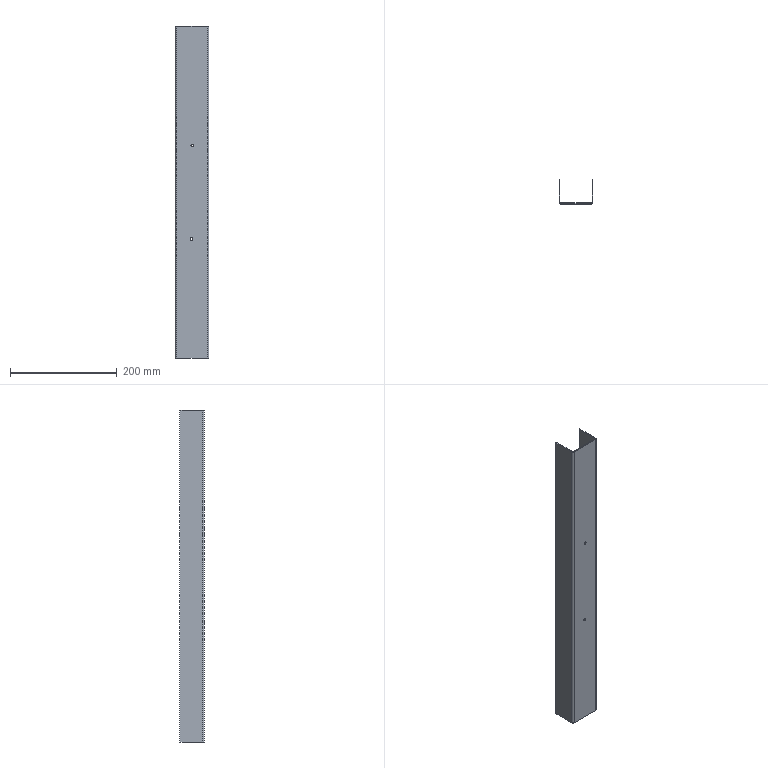Part | SolidWorks | features Cut 1, EdgeFlange 1, FlatPattern 1, SMBaseFlange 1, SheetMetal 1 | 1 solid | 26 faces | box 63 x 45 x 621 mm | volume 137867 mm3 | plane 18 | cylinder 8 | commonest cylinder face diameters 5 x4 3 x2 6 x2
STEP:
#1=CARTESIAN_POINT('',(9.487,-1.5,-176.711));
#2=VERTEX_POINT('',#1);
#3=CARTESIAN_POINT('',(9.487,-1.5,-171.711));
#4=VERTEX_POINT('',#3);
#5=CARTESIAN_POINT('',(9.487,-1.5,-174.211));
#6=DIRECTION('',(0.,1.,0.));
#7=DIRECTION('',(0.,0.,1.));
#8=AXIS2_PLACEMENT_3D('',#5,#6,#7);
#9=CIRCLE('',#8,2.5);
#10=EDGE_CURVE('',#2,#4,#9,.T.);
#11=ORIENTED_EDGE('',*,*,#10,.F.);
#12=CARTESIAN_POINT('',(9.487,0.,-176.711));
#13=VERTEX_POINT('',#12);
#14=CARTESIAN_POINT('',(9.487,-10.,-176.711));
#15=DIRECTION('',(0.,1.,0.));
#16=VECTOR('',#15,1000.);
#17=LINE('',#14,#16);
#18=EDGE_CURVE('',#2,#13,#17,.T.);
#19=ORIENTED_EDGE('',*,*,#18,.T.);
#20=CARTESIAN_POINT('',(9.487,0.,-171.711));
#21=VERTEX_POINT('',#20);
#22=CARTESIAN_POINT('',(9.487,0.,-174.211));
#23=DIRECTION('',(0.,1.,0.));
#24=DIRECTION('',(0.,0.,1.));
#25=AXIS2_PLACEMENT_3D('',#22,#23,#24);
#26=CIRCLE('',#25,2.5);
#27=EDGE_CURVE('',#13,#21,#26,.T.);
#28=ORIENTED_EDGE('',*,*,#27,.T.);
#29=CARTESIAN_POINT('',(9.487,-10.,-171.711));
#30=DIRECTION('',(0.,1.,0.));
#31=VECTOR('',#30,1000.);
#32=LINE('',#29,#31);
#33=EDGE_CURVE('',#4,#21,#32,.T.);
#34=ORIENTED_EDGE('',*,*,#33,.F.);
#35=EDGE_LOOP('',(#11,#19,#28,#34));
#36=FACE_OUTER_BOUND('',#35,.T.);
#37=CARTESIAN_POINT('',(9.487,-10.,-174.211));
#38=DIRECTION('',(0.,1.,0.));
#39=DIRECTION('',(0.,0.,1.));
#40=AXIS2_PLACEMENT_3D('',#37,#38,#39);
#41=CYLINDRICAL_SURFACE('',#40,2.5);
#42=ADVANCED_FACE('',(#36),#41,.F.);
#43=CARTESIAN_POINT('',(8.08,-1.5,-351.711));
#44=VERTEX_POINT('',#43);
#45=CARTESIAN_POINT('',(8.08,-1.5,-346.711));
#46=VERTEX_POINT('',#45);
#47=CARTESIAN_POINT('',(8.08,-1.5,-349.211));
#48=DIRECTION('',(0.,1.,0.));
#49=DIRECTION('',(0.,0.,1.));
#50=AXIS2_PLACEMENT_3D('',#47,#48,#49);
#51=CIRCLE('',#50,2.5);
#52=EDGE_CURVE('',#44,#46,#51,.T.);
#53=ORIENTED_EDGE('',*,*,#52,.F.);
#54=CARTESIAN_POINT('',(8.08,0.,-351.711));
#55=VERTEX_POINT('',#54);
#56=CARTESIAN_POINT('',(8.08,-10.,-351.711));
#57=DIRECTION('',(0.,1.,0.));
#58=VECTOR('',#57,1000.);
#59=LINE('',#56,#58);
#60=EDGE_CURVE('',#44,#55,#59,.T.);
#61=ORIENTED_EDGE('',*,*,#60,.T.);
#62=CARTESIAN_POINT('',(8.08,0.,-346.711));
#63=VERTEX_POINT('',#62);
#64=CARTESIAN_POINT('',(8.08,0.,-349.211));
#65=DIRECTION('',(0.,1.,0.));
#66=DIRECTION('',(0.,0.,1.));
#67=AXIS2_PLACEMENT_3D('',#64,#65,#66);
#68=CIRCLE('',#67,2.5);
#69=EDGE_CURVE('',#55,#63,#68,.T.);
#70=ORIENTED_EDGE('',*,*,#69,.T.);
#71=CARTESIAN_POINT('',(8.08,-10.,-346.711));
#72=DIRECTION('',(0.,1.,0.));
#73=VECTOR('',#72,1000.);
#74=LINE('',#71,#73);
#75=EDGE_CURVE('',#46,#63,#74,.T.);
#76=ORIENTED_EDGE('',*,*,#75,.F.);
#77=EDGE_LOOP('',(#53,#61,#70,#76));
#78=FACE_OUTER_BOUND('',#77,.T.);
#79=CARTESIAN_POINT('',(8.08,-10.,-349.211));
#80=DIRECTION('',(0.,1.,0.));
#81=DIRECTION('',(0.,0.,1.));
#82=AXIS2_PLACEMENT_3D('',#79,#80,#81);
#83=CYLINDRICAL_SURFACE('',#82,2.5);
#84=ADVANCED_FACE('',(#78),#83,.F.);
#85=CARTESIAN_POINT('',(9.487,-1.5,-174.211));
#86=DIRECTION('',(0.,1.,0.));
#87=DIRECTION('',(0.,0.,1.));
#88=AXIS2_PLACEMENT_3D('',#85,#86,#87);
#89=CIRCLE('',#88,2.5);
#90=EDGE_CURVE('',#4,#2,#89,.T.);
#91=ORIENTED_EDGE('',*,*,#90,.T.);
#92=ORIENTED_EDGE('',*,*,#10,.T.);
#93=EDGE_LOOP('',(#91,#92));
#94=FACE_BOUND('',#93,.T.);
#95=CARTESIAN_POINT('',(8.08,-1.5,-349.211));
#96=DIRECTION('',(0.,1.,0.));
#97=DIRECTION('',(0.,0.,1.));
#98=AXIS2_PLACEMENT_3D('',#95,#96,#97);
#99=CIRCLE('',#98,2.5);
#100=EDGE_CURVE('',#46,#44,#99,.T.);
#101=ORIENTED_EDGE('',*,*,#100,.T.);
#102=ORIENTED_EDGE('',*,*,#52,.T.);
#103=EDGE_LOOP('',(#101,#102));
#104=FACE_BOUND('',#103,.T.);
#105=CARTESIAN_POINT('',(37.395,-1.5,-571.611));
#106=VERTEX_POINT('',#105);
#107=CARTESIAN_POINT('',(37.395,-1.5,49.389));
#108=VERTEX_POINT('',#107);
#109=CARTESIAN_POINT('',(37.395,-1.5,-571.611));
#110=DIRECTION('',(0.,0.,1.));
#111=VECTOR('',#110,1000.);
#112=LINE('',#109,#111);
#113=EDGE_CURVE('',#106,#108,#112,.T.);
#114=ORIENTED_EDGE('',*,*,#113,.T.);
#115=CARTESIAN_POINT('',(-19.605,-1.5,49.389));
#116=VERTEX_POINT('',#115);
#117=CARTESIAN_POINT('',(-22.605,-1.5,49.389));
#118=DIRECTION('',(1.,0.,0.));
#119=VECTOR('',#118,1000.);
#120=LINE('',#117,#119);
#121=EDGE_CURVE('',#116,#108,#120,.T.);
#122=ORIENTED_EDGE('',*,*,#121,.F.);
#123=CARTESIAN_POINT('',(-19.605,-1.5,-571.611));
#124=VERTEX_POINT('',#123);
#125=CARTESIAN_POINT('',(-19.605,-1.5,49.389));
#126=DIRECTION('',(0.,0.,-1.));
#127=VECTOR('',#126,1000.);
#128=LINE('',#125,#127);
#129=EDGE_CURVE('',#116,#124,#128,.T.);
#130=ORIENTED_EDGE('',*,*,#129,.T.);
#131=CARTESIAN_POINT('',(-22.605,-1.5,-571.611));
#132=DIRECTION('',(-1.,0.,0.));
#133=VECTOR('',#132,1000.);
#134=LINE('',#131,#133);
#135=EDGE_CURVE('',#106,#124,#134,.T.);
#136=ORIENTED_EDGE('',*,*,#135,.F.);
#137=EDGE_LOOP('',(#114,#122,#130,#136));
#138=FACE_OUTER_BOUND('',#137,.T.);
#139=CARTESIAN_POINT('',(0.,-1.5,0.));
#140=DIRECTION('',(0.,1.,0.));
#141=DIRECTION('',(0.,0.,1.));
#142=AXIS2_PLACEMENT_3D('',#139,#140,#141);
#143=PLANE('',#142);
#144=ADVANCED_FACE('',(#94,#104,#138),#143,.F.);
#145=CARTESIAN_POINT('',(9.487,0.,-174.211));
#146=DIRECTION('',(0.,1.,0.));
#147=DIRECTION('',(0.,0.,1.));
#148=AXIS2_PLACEMENT_3D('',#145,#146,#147);
#149=CIRCLE('',#148,2.5);
#150=EDGE_CURVE('',#21,#13,#149,.T.);
#151=ORIENTED_EDGE('',*,*,#150,.F.);
#152=ORIENTED_EDGE('',*,*,#27,.F.);
#153=EDGE_LOOP('',(#151,#152));
#154=FACE_BOUND('',#153,.T.);
#155=CARTESIAN_POINT('',(8.08,0.,-349.211));
#156=DIRECTION('',(0.,1.,0.));
#157=DIRECTION('',(0.,0.,1.));
#158=AXIS2_PLACEMENT_3D('',#155,#156,#157);
#159=CIRCLE('',#158,2.5);
#160=EDGE_CURVE('',#63,#55,#159,.T.);
#161=ORIENTED_EDGE('',*,*,#160,.F.);
#162=ORIENTED_EDGE('',*,*,#69,.F.);
#163=EDGE_LOOP('',(#161,#162));
#164=FACE_BOUND('',#163,.T.);
#165=CARTESIAN_POINT('',(-19.605,0.,49.389));
#166=VERTEX_POINT('',#165);
#167=CARTESIAN_POINT('',(37.395,0.,49.389));
#168=VERTEX_POINT('',#167);
#169=CARTESIAN_POINT('',(-22.605,0.,49.389));
#170=DIRECTION('',(1.,0.,0.));
#171=VECTOR('',#170,1000.);
#172=LINE('',#169,#171);
#173=EDGE_CURVE('',#166,#168,#172,.T.);
#174=ORIENTED_EDGE('',*,*,#173,.T.);
#175=CARTESIAN_POINT('',(37.395,0.,-571.611));
#176=VERTEX_POINT('',#175);
#177=CARTESIAN_POINT('',(37.395,0.,-571.611));
#178=DIRECTION('',(0.,0.,1.));
#179=VECTOR('',#178,1000.);
#180=LINE('',#177,#179);
#181=EDGE_CURVE('',#176,#168,#180,.T.);
#182=ORIENTED_EDGE('',*,*,#181,.F.);
#183=CARTESIAN_POINT('',(-19.605,0.,-571.611));
#184=VERTEX_POINT('',#183);
#185=CARTESIAN_POINT('',(-22.605,0.,-571.611));
#186=DIRECTION('',(-1.,0.,0.));
#187=VECTOR('',#186,1000.);
#188=LINE('',#185,#187);
#189=EDGE_CURVE('',#176,#184,#188,.T.);
#190=ORIENTED_EDGE('',*,*,#189,.T.);
#191=CARTESIAN_POINT('',(-19.605,0.,49.389));
#192=DIRECTION('',(0.,0.,-1.));
#193=VECTOR('',#192,1000.);
#194=LINE('',#191,#193);
#195=EDGE_CURVE('',#166,#184,#194,.T.);
#196=ORIENTED_EDGE('',*,*,#195,.F.);
#197=EDGE_LOOP('',(#174,#182,#190,#196));
#198=FACE_OUTER_BOUND('',#197,.T.);
#199=CARTESIAN_POINT('',(0.,0.,0.));
#200=DIRECTION('',(0.,1.,0.));
#201=DIRECTION('',(0.,0.,1.));
#202=AXIS2_PLACEMENT_3D('',#199,#200,#201);
#203=PLANE('',#202);
#204=ADVANCED_FACE('',(#154,#164,#198),#203,.T.);
#205=ORIENTED_EDGE('',*,*,#189,.F.);
#206=CARTESIAN_POINT('',(37.395,0.,-571.611));
#207=DIRECTION('',(0.,-1.,0.));
#208=VECTOR('',#207,1000.);
#209=LINE('',#206,#208);
#210=EDGE_CURVE('',#176,#106,#209,.T.);
#211=ORIENTED_EDGE('',*,*,#210,.T.);
#212=ORIENTED_EDGE('',*,*,#135,.T.);
#213=CARTESIAN_POINT('',(-19.605,0.,-571.611));
#214=DIRECTION('',(0.,-1.,0.));
#215=VECTOR('',#214,1000.);
#216=LINE('',#213,#215);
#217=EDGE_CURVE('',#184,#124,#216,.T.);
#218=ORIENTED_EDGE('',*,*,#217,.F.);
#219=EDGE_LOOP('',(#205,#211,#212,#218));
#220=FACE_OUTER_BOUND('',#219,.T.);
#221=CARTESIAN_POINT('',(-22.605,-1.5,-571.611));
#222=DIRECTION('',(0.,0.,-1.));
#223=DIRECTION('',(-1.,0.,0.));
#224=AXIS2_PLACEMENT_3D('',#221,#222,#223);
#225=PLANE('',#224);
#226=ADVANCED_FACE('',(#220),#225,.T.);
#227=CARTESIAN_POINT('',(37.395,0.,49.389));
#228=DIRECTION('',(0.,-1.,0.));
#229=VECTOR('',#228,1000.);
#230=LINE('',#227,#229);
#231=EDGE_CURVE('',#168,#108,#230,.T.);
#232=ORIENTED_EDGE('',*,*,#231,.F.);
#233=ORIENTED_EDGE('',*,*,#173,.F.);
#234=CARTESIAN_POINT('',(-19.605,0.,49.389));
#235=DIRECTION('',(0.,-1.,0.));
#236=VECTOR('',#235,1000.);
#237=LINE('',#234,#236);
#238=EDGE_CURVE('',#166,#116,#237,.T.);
#239=ORIENTED_EDGE('',*,*,#238,.T.);
#240=ORIENTED_EDGE('',*,*,#121,.T.);
#241=EDGE_LOOP('',(#232,#233,#239,#240));
#242=FACE_OUTER_BOUND('',#241,.T.);
#243=CARTESIAN_POINT('',(-22.605,-1.5,49.389));
#244=DIRECTION('',(0.,0.,1.));
#245=DIRECTION('',(1.,0.,0.));
#246=AXIS2_PLACEMENT_3D('',#243,#244,#245);
#247=PLANE('',#246);
#248=ADVANCED_FACE('',(#242),#247,.T.);
#249=CARTESIAN_POINT('',(-21.105,1.5,-571.611));
#250=VERTEX_POINT('',#249);
#251=CARTESIAN_POINT('',(-22.605,1.5,-571.611));
#252=VERTEX_POINT('',#251);
#253=CARTESIAN_POINT('',(-22.605,1.5,-571.611));
#254=DIRECTION('',(-1.,0.,0.));
#255=VECTOR('',#254,1000.);
#256=LINE('',#253,#255);
#257=EDGE_CURVE('',#250,#252,#256,.T.);
#258=ORIENTED_EDGE('',*,*,#257,.F.);
#259=CARTESIAN_POINT('',(-19.605,1.5,-571.611));
#260=DIRECTION('',(0.,0.,-1.));
#261=DIRECTION('',(1.,0.,0.));
#262=AXIS2_PLACEMENT_3D('',#259,#260,#261);
#263=CIRCLE('',#262,1.5);
#264=EDGE_CURVE('',#184,#250,#263,.T.);
#265=ORIENTED_EDGE('',*,*,#264,.F.);
#266=ORIENTED_EDGE('',*,*,#217,.T.);
#267=CARTESIAN_POINT('',(-19.605,1.5,-571.611));
#268=DIRECTION('',(0.,0.,-1.));
#269=DIRECTION('',(1.,0.,0.));
#270=AXIS2_PLACEMENT_3D('',#267,#268,#269);
#271=CIRCLE('',#270,3.);
#272=EDGE_CURVE('',#124,#252,#271,.T.);
#273=ORIENTED_EDGE('',*,*,#272,.T.);
#274=EDGE_LOOP('',(#258,#265,#266,#273));
#275=FACE_OUTER_BOUND('',#274,.T.);
#276=CARTESIAN_POINT('',(-19.605,1.5,-571.611));
#277=DIRECTION('',(0.,0.,-1.));
#278=DIRECTION('',(-1.,0.,0.));
#279=AXIS2_PLACEMENT_3D('',#276,#277,#278);
#280=PLANE('',#279);
#281=ADVANCED_FACE('',(#275),#280,.T.);
#282=CARTESIAN_POINT('',(-21.105,1.5,49.389));
#283=VERTEX_POINT('',#282);
#284=CARTESIAN_POINT('',(-19.605,1.5,49.389));
#285=DIRECTION('',(0.,0.,1.));
#286=DIRECTION('',(1.,0.,0.));
#287=AXIS2_PLACEMENT_3D('',#284,#285,#286);
#288=CIRCLE('',#287,1.5);
#289=EDGE_CURVE('',#283,#166,#288,.T.);
#290=ORIENTED_EDGE('',*,*,#289,.F.);
#291=CARTESIAN_POINT('',(-22.605,1.5,49.389));
#292=VERTEX_POINT('',#291);
#293=CARTESIAN_POINT('',(-21.105,1.5,49.389));
#294=DIRECTION('',(-1.,0.,0.));
#295=VECTOR('',#294,1000.);
#296=LINE('',#293,#295);
#297=EDGE_CURVE('',#283,#292,#296,.T.);
#298=ORIENTED_EDGE('',*,*,#297,.T.);
#299=CARTESIAN_POINT('',(-19.605,1.5,49.389));
#300=DIRECTION('',(0.,0.,1.));
#301=DIRECTION('',(1.,0.,0.));
#302=AXIS2_PLACEMENT_3D('',#299,#300,#301);
#303=CIRCLE('',#302,3.);
#304=EDGE_CURVE('',#292,#116,#303,.T.);
#305=ORIENTED_EDGE('',*,*,#304,.T.);
#306=ORIENTED_EDGE('',*,*,#238,.F.);
#307=EDGE_LOOP('',(#290,#298,#305,#306));
#308=FACE_OUTER_BOUND('',#307,.T.);
#309=CARTESIAN_POINT('',(-19.605,1.5,49.389));
#310=DIRECTION('',(0.,0.,-1.));
#311=DIRECTION('',(-1.,0.,0.));
#312=AXIS2_PLACEMENT_3D('',#309,#310,#311);
#313=PLANE('',#312);
#314=ADVANCED_FACE('',(#308),#313,.F.);
#315=ORIENTED_EDGE('',*,*,#129,.F.);
#316=ORIENTED_EDGE('',*,*,#304,.F.);
#317=CARTESIAN_POINT('',(-22.605,1.5,-571.611));
#318=DIRECTION('',(0.,0.,-1.));
#319=VECTOR('',#318,1000.);
#320=LINE('',#317,#319);
#321=EDGE_CURVE('',#292,#252,#320,.T.);
#322=ORIENTED_EDGE('',*,*,#321,.T.);
#323=ORIENTED_EDGE('',*,*,#272,.F.);
#324=EDGE_LOOP('',(#315,#316,#322,#323));
#325=FACE_OUTER_BOUND('',#324,.T.);
#326=CARTESIAN_POINT('',(-19.605,1.5,49.389));
#327=DIRECTION('',(0.,0.,1.));
#328=DIRECTION('',(-1.,0.,0.));
#329=AXIS2_PLACEMENT_3D('',#326,#327,#328);
#330=CYLINDRICAL_SURFACE('',#329,3.);
#331=ADVANCED_FACE('',(#325),#330,.T.);
#332=ORIENTED_EDGE('',*,*,#195,.T.);
#333=ORIENTED_EDGE('',*,*,#264,.T.);
#334=CARTESIAN_POINT('',(-21.105,1.5,-571.611));
#335=DIRECTION('',(0.,0.,1.));
#336=VECTOR('',#335,1000.);
#337=LINE('',#334,#336);
#338=EDGE_CURVE('',#250,#283,#337,.T.);
#339=ORIENTED_EDGE('',*,*,#338,.T.);
#340=ORIENTED_EDGE('',*,*,#289,.T.);
#341=EDGE_LOOP('',(#332,#333,#339,#340));
#342=FACE_OUTER_BOUND('',#341,.T.);
#343=CARTESIAN_POINT('',(-19.605,1.5,49.389));
#344=DIRECTION('',(0.,0.,1.));
#345=DIRECTION('',(-1.,0.,0.));
#346=AXIS2_PLACEMENT_3D('',#343,#344,#345);
#347=CYLINDRICAL_SURFACE('',#346,1.5);
#348=ADVANCED_FACE('',(#342),#347,.F.);
#349=ORIENTED_EDGE('',*,*,#257,.T.);
#350=CARTESIAN_POINT('',(-22.605,43.5,-571.611));
#351=VERTEX_POINT('',#350);
#352=CARTESIAN_POINT('',(-22.605,0.,-571.611));
#353=DIRECTION('',(0.,-1.,0.));
#354=VECTOR('',#353,1000.);
#355=LINE('',#352,#354);
#356=EDGE_CURVE('',#351,#252,#355,.T.);
#357=ORIENTED_EDGE('',*,*,#356,.F.);
#358=CARTESIAN_POINT('',(-21.105,43.5,-571.611));
#359=VERTEX_POINT('',#358);
#360=CARTESIAN_POINT('',(-22.605,43.5,-571.611));
#361=DIRECTION('',(1.,0.,0.));
#362=VECTOR('',#361,1000.);
#363=LINE('',#360,#362);
#364=EDGE_CURVE('',#351,#359,#363,.T.);
#365=ORIENTED_EDGE('',*,*,#364,.T.);
#366=CARTESIAN_POINT('',(-21.105,0.,-571.611));
#367=DIRECTION('',(0.,-1.,0.));
#368=VECTOR('',#367,1000.);
#369=LINE('',#366,#368);
#370=EDGE_CURVE('',#359,#250,#369,.T.);
#371=ORIENTED_EDGE('',*,*,#370,.T.);
#372=EDGE_LOOP('',(#349,#357,#365,#371));
#373=FACE_OUTER_BOUND('',#372,.T.);
#374=CARTESIAN_POINT('',(-22.605,0.,-571.611));
#375=DIRECTION('',(0.,0.,1.));
#376=DIRECTION('',(1.,0.,0.));
#377=AXIS2_PLACEMENT_3D('',#374,#375,#376);
#378=PLANE('',#377);
#379=ADVANCED_FACE('',(#373),#378,.F.);
#380=ORIENTED_EDGE('',*,*,#297,.F.);
#381=CARTESIAN_POINT('',(-21.105,43.5,49.389));
#382=VERTEX_POINT('',#381);
#383=CARTESIAN_POINT('',(-21.105,43.5,49.389));
#384=DIRECTION('',(0.,1.,0.));
#385=VECTOR('',#384,1000.);
#386=LINE('',#383,#385);
#387=EDGE_CURVE('',#283,#382,#386,.T.);
#388=ORIENTED_EDGE('',*,*,#387,.T.);
#389=CARTESIAN_POINT('',(-22.605,43.5,49.389));
#390=VERTEX_POINT('',#389);
#391=CARTESIAN_POINT('',(-22.605,43.5,49.389));
#392=DIRECTION('',(1.,0.,0.));
#393=VECTOR('',#392,1000.);
#394=LINE('',#391,#393);
#395=EDGE_CURVE('',#390,#382,#394,.T.);
#396=ORIENTED_EDGE('',*,*,#395,.F.);
#397=CARTESIAN_POINT('',(-22.605,0.,49.389));
#398=DIRECTION('',(0.,1.,0.));
#399=VECTOR('',#398,1000.);
#400=LINE('',#397,#399);
#401=EDGE_CURVE('',#292,#390,#400,.T.);
#402=ORIENTED_EDGE('',*,*,#401,.F.);
#403=EDGE_LOOP('',(#380,#388,#396,#402));
#404=FACE_OUTER_BOUND('',#403,.T.);
#405=CARTESIAN_POINT('',(-22.605,43.5,49.389));
#406=DIRECTION('',(0.,0.,-1.));
#407=DIRECTION('',(-1.,0.,0.));
#408=AXIS2_PLACEMENT_3D('',#405,#406,#407);
#409=PLANE('',#408);
#410=ADVANCED_FACE('',(#404),#409,.F.);
#411=ORIENTED_EDGE('',*,*,#321,.F.);
#412=ORIENTED_EDGE('',*,*,#401,.T.);
#413=CARTESIAN_POINT('',(-22.605,43.5,0.));
#414=DIRECTION('',(0.,0.,-1.));
#415=VECTOR('',#414,1000.);
#416=LINE('',#413,#415);
#417=EDGE_CURVE('',#390,#351,#416,.T.);
#418=ORIENTED_EDGE('',*,*,#417,.T.);
#419=ORIENTED_EDGE('',*,*,#356,.T.);
#420=EDGE_LOOP('',(#411,#412,#418,#419));
#421=FACE_OUTER_BOUND('',#420,.T.);
#422=CARTESIAN_POINT('',(-22.605,0.,0.));
#423=DIRECTION('',(1.,0.,0.));
#424=DIRECTION('',(0.,1.,0.));
#425=AXIS2_PLACEMENT_3D('',#422,#423,#424);
#426=PLANE('',#425);
#427=ADVANCED_FACE('',(#421),#426,.F.);
#428=ORIENTED_EDGE('',*,*,#387,.F.);
#429=ORIENTED_EDGE('',*,*,#338,.F.);
#430=ORIENTED_EDGE('',*,*,#370,.F.);
#431=CARTESIAN_POINT('',(-21.105,43.5,-571.611));
#432=DIRECTION('',(0.,0.,-1.));
#433=VECTOR('',#432,1000.);
#434=LINE('',#431,#433);
#435=EDGE_CURVE('',#382,#359,#434,.T.);
#436=ORIENTED_EDGE('',*,*,#435,.F.);
#437=EDGE_LOOP('',(#428,#429,#430,#436));
#438=FACE_OUTER_BOUND('',#437,.T.);
#439=CARTESIAN_POINT('',(-21.105,0.,0.));
#440=DIRECTION('',(1.,0.,0.));
#441=DIRECTION('',(0.,1.,0.));
#442=AXIS2_PLACEMENT_3D('',#439,#440,#441);
#443=PLANE('',#442);
#444=ADVANCED_FACE('',(#438),#443,.T.);
#445=ORIENTED_EDGE('',*,*,#435,.T.);
#446=ORIENTED_EDGE('',*,*,#364,.F.);
#447=ORIENTED_EDGE('',*,*,#417,.F.);
#448=ORIENTED_EDGE('',*,*,#395,.T.);
#449=EDGE_LOOP('',(#445,#446,#447,#448));
#450=FACE_OUTER_BOUND('',#449,.T.);
#451=CARTESIAN_POINT('',(-22.605,43.5,-571.611));
#452=DIRECTION('',(0.,-1.,0.));
#453=DIRECTION('',(1.,0.,0.));
#454=AXIS2_PLACEMENT_3D('',#451,#452,#453);
#455=PLANE('',#454);
#456=ADVANCED_FACE('',(#450),#455,.F.);
#457=CARTESIAN_POINT('',(38.895,1.5,49.389));
#458=VERTEX_POINT('',#457);
#459=CARTESIAN_POINT('',(40.395,1.5,49.389));
#460=VERTEX_POINT('',#459);
#461=CARTESIAN_POINT('',(40.395,1.5,49.389));
#462=DIRECTION('',(1.,0.,0.));
#463=VECTOR('',#462,1000.);
#464=LINE('',#461,#463);
#465=EDGE_CURVE('',#458,#460,#464,.T.);
#466=ORIENTED_EDGE('',*,*,#465,.F.);
#467=CARTESIAN_POINT('',(37.395,1.5,49.389));
#468=DIRECTION('',(0.,0.,1.));
#469=DIRECTION('',(0.,1.,0.));
#470=AXIS2_PLACEMENT_3D('',#467,#468,#469);
#471=CIRCLE('',#470,1.5);
#472=EDGE_CURVE('',#168,#458,#471,.T.);
#473=ORIENTED_EDGE('',*,*,#472,.F.);
#474=ORIENTED_EDGE('',*,*,#231,.T.);
#475=CARTESIAN_POINT('',(37.395,1.5,49.389));
#476=DIRECTION('',(0.,0.,1.));
#477=DIRECTION('',(0.,1.,0.));
#478=AXIS2_PLACEMENT_3D('',#475,#476,#477);
#479=CIRCLE('',#478,3.);
#480=EDGE_CURVE('',#108,#460,#479,.T.);
#481=ORIENTED_EDGE('',*,*,#480,.T.);
#482=EDGE_LOOP('',(#466,#473,#474,#481));
#483=FACE_OUTER_BOUND('',#482,.T.);
#484=CARTESIAN_POINT('',(37.395,1.5,49.389));
#485=DIRECTION('',(0.,0.,1.));
#486=DIRECTION('',(0.,-1.,0.));
#487=AXIS2_PLACEMENT_3D('',#484,#485,#486);
#488=PLANE('',#487);
#489=ADVANCED_FACE('',(#483),#488,.T.);
#490=CARTESIAN_POINT('',(38.895,1.5,-571.611));
#491=VERTEX_POINT('',#490);
#492=CARTESIAN_POINT('',(37.395,1.5,-571.611));
#493=DIRECTION('',(0.,0.,-1.));
#494=DIRECTION('',(0.,1.,0.));
#495=AXIS2_PLACEMENT_3D('',#492,#493,#494);
#496=CIRCLE('',#495,1.5);
#497=EDGE_CURVE('',#491,#176,#496,.T.);
#498=ORIENTED_EDGE('',*,*,#497,.F.);
#499=CARTESIAN_POINT('',(40.395,1.5,-571.611));
#500=VERTEX_POINT('',#499);
#501=CARTESIAN_POINT('',(38.895,1.5,-571.611));
#502=DIRECTION('',(1.,0.,0.));
#503=VECTOR('',#502,1000.);
#504=LINE('',#501,#503);
#505=EDGE_CURVE('',#491,#500,#504,.T.);
#506=ORIENTED_EDGE('',*,*,#505,.T.);
#507=CARTESIAN_POINT('',(37.395,1.5,-571.611));
#508=DIRECTION('',(0.,0.,-1.));
#509=DIRECTION('',(0.,1.,0.));
#510=AXIS2_PLACEMENT_3D('',#507,#508,#509);
#511=CIRCLE('',#510,3.);
#512=EDGE_CURVE('',#500,#106,#511,.T.);
#513=ORIENTED_EDGE('',*,*,#512,.T.);
#514=ORIENTED_EDGE('',*,*,#210,.F.);
#515=EDGE_LOOP('',(#498,#506,#513,#514));
#516=FACE_OUTER_BOUND('',#515,.T.);
#517=CARTESIAN_POINT('',(37.395,1.5,-571.611));
#518=DIRECTION('',(0.,0.,1.));
#519=DIRECTION('',(0.,-1.,0.));
#520=AXIS2_PLACEMENT_3D('',#517,#518,#519);
#521=PLANE('',#520);
#522=ADVANCED_FACE('',(#516),#521,.F.);
#523=ORIENTED_EDGE('',*,*,#113,.F.);
#524=ORIENTED_EDGE('',*,*,#512,.F.);
#525=CARTESIAN_POINT('',(40.395,1.5,49.389));
#526=DIRECTION('',(0.,0.,1.));
#527=VECTOR('',#526,1000.);
#528=LINE('',#525,#527);
#529=EDGE_CURVE('',#500,#460,#528,.T.);
#530=ORIENTED_EDGE('',*,*,#529,.T.);
#531=ORIENTED_EDGE('',*,*,#480,.F.);
#532=EDGE_LOOP('',(#523,#524,#530,#531));
#533=FACE_OUTER_BOUND('',#532,.T.);
#534=CARTESIAN_POINT('',(37.395,1.5,-571.611));
#535=DIRECTION('',(0.,0.,-1.));
#536=DIRECTION('',(1.,0.,0.));
#537=AXIS2_PLACEMENT_3D('',#534,#535,#536);
#538=CYLINDRICAL_SURFACE('',#537,3.);
#539=ADVANCED_FACE('',(#533),#538,.T.);
#540=ORIENTED_EDGE('',*,*,#181,.T.);
#541=ORIENTED_EDGE('',*,*,#472,.T.);
#542=CARTESIAN_POINT('',(38.895,1.5,49.389));
#543=DIRECTION('',(0.,0.,-1.));
#544=VECTOR('',#543,1000.);
#545=LINE('',#542,#544);
#546=EDGE_CURVE('',#458,#491,#545,.T.);
#547=ORIENTED_EDGE('',*,*,#546,.T.);
#548=ORIENTED_EDGE('',*,*,#497,.T.);
#549=EDGE_LOOP('',(#540,#541,#547,#548));
#550=FACE_OUTER_BOUND('',#549,.T.);
#551=CARTESIAN_POINT('',(37.395,1.5,-571.611));
#552=DIRECTION('',(0.,0.,-1.));
#553=DIRECTION('',(1.,0.,0.));
#554=AXIS2_PLACEMENT_3D('',#551,#552,#553);
#555=CYLINDRICAL_SURFACE('',#554,1.5);
#556=ADVANCED_FACE('',(#550),#555,.F.);
#557=ORIENTED_EDGE('',*,*,#465,.T.);
#558=CARTESIAN_POINT('',(40.395,43.5,49.389));
#559=VERTEX_POINT('',#558);
#560=CARTESIAN_POINT('',(40.395,0.,49.389));
#561=DIRECTION('',(0.,-1.,0.));
#562=VECTOR('',#561,1000.);
#563=LINE('',#560,#562);
#564=EDGE_CURVE('',#559,#460,#563,.T.);
#565=ORIENTED_EDGE('',*,*,#564,.F.);
#566=CARTESIAN_POINT('',(38.895,43.5,49.389));
#567=VERTEX_POINT('',#566);
#568=CARTESIAN_POINT('',(40.395,43.5,49.389));
#569=DIRECTION('',(-1.,0.,0.));
#570=VECTOR('',#569,1000.);
#571=LINE('',#568,#570);
#572=EDGE_CURVE('',#559,#567,#571,.T.);
#573=ORIENTED_EDGE('',*,*,#572,.T.);
#574=CARTESIAN_POINT('',(38.895,0.,49.389));
#575=DIRECTION('',(0.,-1.,0.));
#576=VECTOR('',#575,1000.);
#577=LINE('',#574,#576);
#578=EDGE_CURVE('',#567,#458,#577,.T.);
#579=ORIENTED_EDGE('',*,*,#578,.T.);
#580=EDGE_LOOP('',(#557,#565,#573,#579));
#581=FACE_OUTER_BOUND('',#580,.T.);
#582=CARTESIAN_POINT('',(40.395,0.,49.389));
#583=DIRECTION('',(0.,0.,-1.));
#584=DIRECTION('',(0.,1.,0.));
#585=AXIS2_PLACEMENT_3D('',#582,#583,#584);
#586=PLANE('',#585);
#587=ADVANCED_FACE('',(#581),#586,.F.);
#588=ORIENTED_EDGE('',*,*,#505,.F.);
#589=CARTESIAN_POINT('',(38.895,43.5,-571.611));
#590=VERTEX_POINT('',#589);
#591=CARTESIAN_POINT('',(38.895,43.5,-571.611));
#592=DIRECTION('',(0.,1.,0.));
#593=VECTOR('',#592,1000.);
#594=LINE('',#591,#593);
#595=EDGE_CURVE('',#491,#590,#594,.T.);
#596=ORIENTED_EDGE('',*,*,#595,.T.);
#597=CARTESIAN_POINT('',(40.395,43.5,-571.611));
#598=VERTEX_POINT('',#597);
#599=CARTESIAN_POINT('',(40.395,43.5,-571.611));
#600=DIRECTION('',(-1.,0.,0.));
#601=VECTOR('',#600,1000.);
#602=LINE('',#599,#601);
#603=EDGE_CURVE('',#598,#590,#602,.T.);
#604=ORIENTED_EDGE('',*,*,#603,.F.);
#605=CARTESIAN_POINT('',(40.395,0.,-571.611));
#606=DIRECTION('',(0.,1.,0.));
#607=VECTOR('',#606,1000.);
#608=LINE('',#605,#607);
#609=EDGE_CURVE('',#500,#598,#608,.T.);
#610=ORIENTED_EDGE('',*,*,#609,.F.);
#611=EDGE_LOOP('',(#588,#596,#604,#610));
#612=FACE_OUTER_BOUND('',#611,.T.);
#613=CARTESIAN_POINT('',(40.395,43.5,-571.611));
#614=DIRECTION('',(0.,0.,1.));
#615=DIRECTION('',(1.,0.,0.));
#616=AXIS2_PLACEMENT_3D('',#613,#614,#615);
#617=PLANE('',#616);
#618=ADVANCED_FACE('',(#612),#617,.F.);
#619=ORIENTED_EDGE('',*,*,#529,.F.);
#620=ORIENTED_EDGE('',*,*,#609,.T.);
#621=CARTESIAN_POINT('',(40.395,43.5,0.));
#622=DIRECTION('',(0.,0.,1.));
#623=VECTOR('',#622,1000.);
#624=LINE('',#621,#623);
#625=EDGE_CURVE('',#598,#559,#624,.T.);
#626=ORIENTED_EDGE('',*,*,#625,.T.);
#627=ORIENTED_EDGE('',*,*,#564,.T.);
#628=EDGE_LOOP('',(#619,#620,#626,#627));
#629=FACE_OUTER_BOUND('',#628,.T.);
#630=CARTESIAN_POINT('',(40.395,0.,0.));
#631=DIRECTION('',(-1.,0.,0.));
#632=DIRECTION('',(0.,-1.,0.));
#633=AXIS2_PLACEMENT_3D('',#630,#631,#632);
#634=PLANE('',#633);
#635=ADVANCED_FACE('',(#629),#634,.F.);
#636=ORIENTED_EDGE('',*,*,#595,.F.);
#637=ORIENTED_EDGE('',*,*,#546,.F.);
#638=ORIENTED_EDGE('',*,*,#578,.F.);
#639=CARTESIAN_POINT('',(38.895,43.5,49.389));
#640=DIRECTION('',(0.,0.,1.));
#641=VECTOR('',#640,1000.);
#642=LINE('',#639,#641);
#643=EDGE_CURVE('',#590,#567,#642,.T.);
#644=ORIENTED_EDGE('',*,*,#643,.F.);
#645=EDGE_LOOP('',(#636,#637,#638,#644));
#646=FACE_OUTER_BOUND('',#645,.T.);
#647=CARTESIAN_POINT('',(38.895,0.,0.));
#648=DIRECTION('',(-1.,0.,0.));
#649=DIRECTION('',(0.,-1.,0.));
#650=AXIS2_PLACEMENT_3D('',#647,#648,#649);
#651=PLANE('',#650);
#652=ADVANCED_FACE('',(#646),#651,.T.);
#653=ORIENTED_EDGE('',*,*,#643,.T.);
#654=ORIENTED_EDGE('',*,*,#572,.F.);
#655=ORIENTED_EDGE('',*,*,#625,.F.);
#656=ORIENTED_EDGE('',*,*,#603,.T.);
#657=EDGE_LOOP('',(#653,#654,#655,#656));
#658=FACE_OUTER_BOUND('',#657,.T.);
#659=CARTESIAN_POINT('',(40.395,43.5,49.389));
#660=DIRECTION('',(0.,-1.,0.));
#661=DIRECTION('',(1.,0.,0.));
#662=AXIS2_PLACEMENT_3D('',#659,#660,#661);
#663=PLANE('',#662);
#664=ADVANCED_FACE('',(#658),#663,.F.);
#665=ORIENTED_EDGE('',*,*,#60,.F.);
#666=ORIENTED_EDGE('',*,*,#100,.F.);
#667=ORIENTED_EDGE('',*,*,#75,.T.);
#668=ORIENTED_EDGE('',*,*,#160,.T.);
#669=EDGE_LOOP('',(#665,#666,#667,#668));
#670=FACE_OUTER_BOUND('',#669,.T.);
#671=CARTESIAN_POINT('',(8.08,-10.,-349.211));
#672=DIRECTION('',(0.,1.,0.));
#673=DIRECTION('',(0.,0.,1.));
#674=AXIS2_PLACEMENT_3D('',#671,#672,#673);
#675=CYLINDRICAL_SURFACE('',#674,2.5);
#676=ADVANCED_FACE('',(#670),#675,.F.);
#677=ORIENTED_EDGE('',*,*,#18,.F.);
#678=ORIENTED_EDGE('',*,*,#90,.F.);
#679=ORIENTED_EDGE('',*,*,#33,.T.);
#680=ORIENTED_EDGE('',*,*,#150,.T.);
#681=EDGE_LOOP('',(#677,#678,#679,#680));
#682=FACE_OUTER_BOUND('',#681,.T.);
#683=CARTESIAN_POINT('',(9.487,-10.,-174.211));
#684=DIRECTION('',(0.,1.,0.));
#685=DIRECTION('',(0.,0.,1.));
#686=AXIS2_PLACEMENT_3D('',#683,#684,#685);
#687=CYLINDRICAL_SURFACE('',#686,2.5);
#688=ADVANCED_FACE('',(#682),#687,.F.);
#689=CLOSED_SHELL('',(#42,#84,#144,#204,#226,#248,#281,#314,#331,#348,#379,#410,#427,#444,#456,#489,#522,#539,#556,#587,#618,#635,#652,#664,#676,#688));
#690=MANIFOLD_SOLID_BREP('',#689);
#691=CARTESIAN_POINT('',(0.,0.,0.));
#692=DIRECTION('',(0.,0.,1.));
#693=DIRECTION('',(1.,0.,0.));
#694=AXIS2_PLACEMENT_3D('',#691,#692,#693);
#695=(LENGTH_UNIT()NAMED_UNIT(*)SI_UNIT(.MILLI.,.METRE.));
#696=UNCERTAINTY_MEASURE_WITH_UNIT(LENGTH_MEASURE(0.00001),#695,'','');
#697=(NAMED_UNIT(*)PLANE_ANGLE_UNIT()SI_UNIT($,.RADIAN.));
#698=(NAMED_UNIT(*)SI_UNIT($,.STERADIAN.)SOLID_ANGLE_UNIT());
#699=(GEOMETRIC_REPRESENTATION_CONTEXT(3)GLOBAL_UNCERTAINTY_ASSIGNED_CONTEXT((#696))GLOBAL_UNIT_ASSIGNED_CONTEXT((#695,#697,#698))REPRESENTATION_CONTEXT('',''));
#700=ADVANCED_BREP_SHAPE_REPRESENTATION('',(#690,#694),#699);